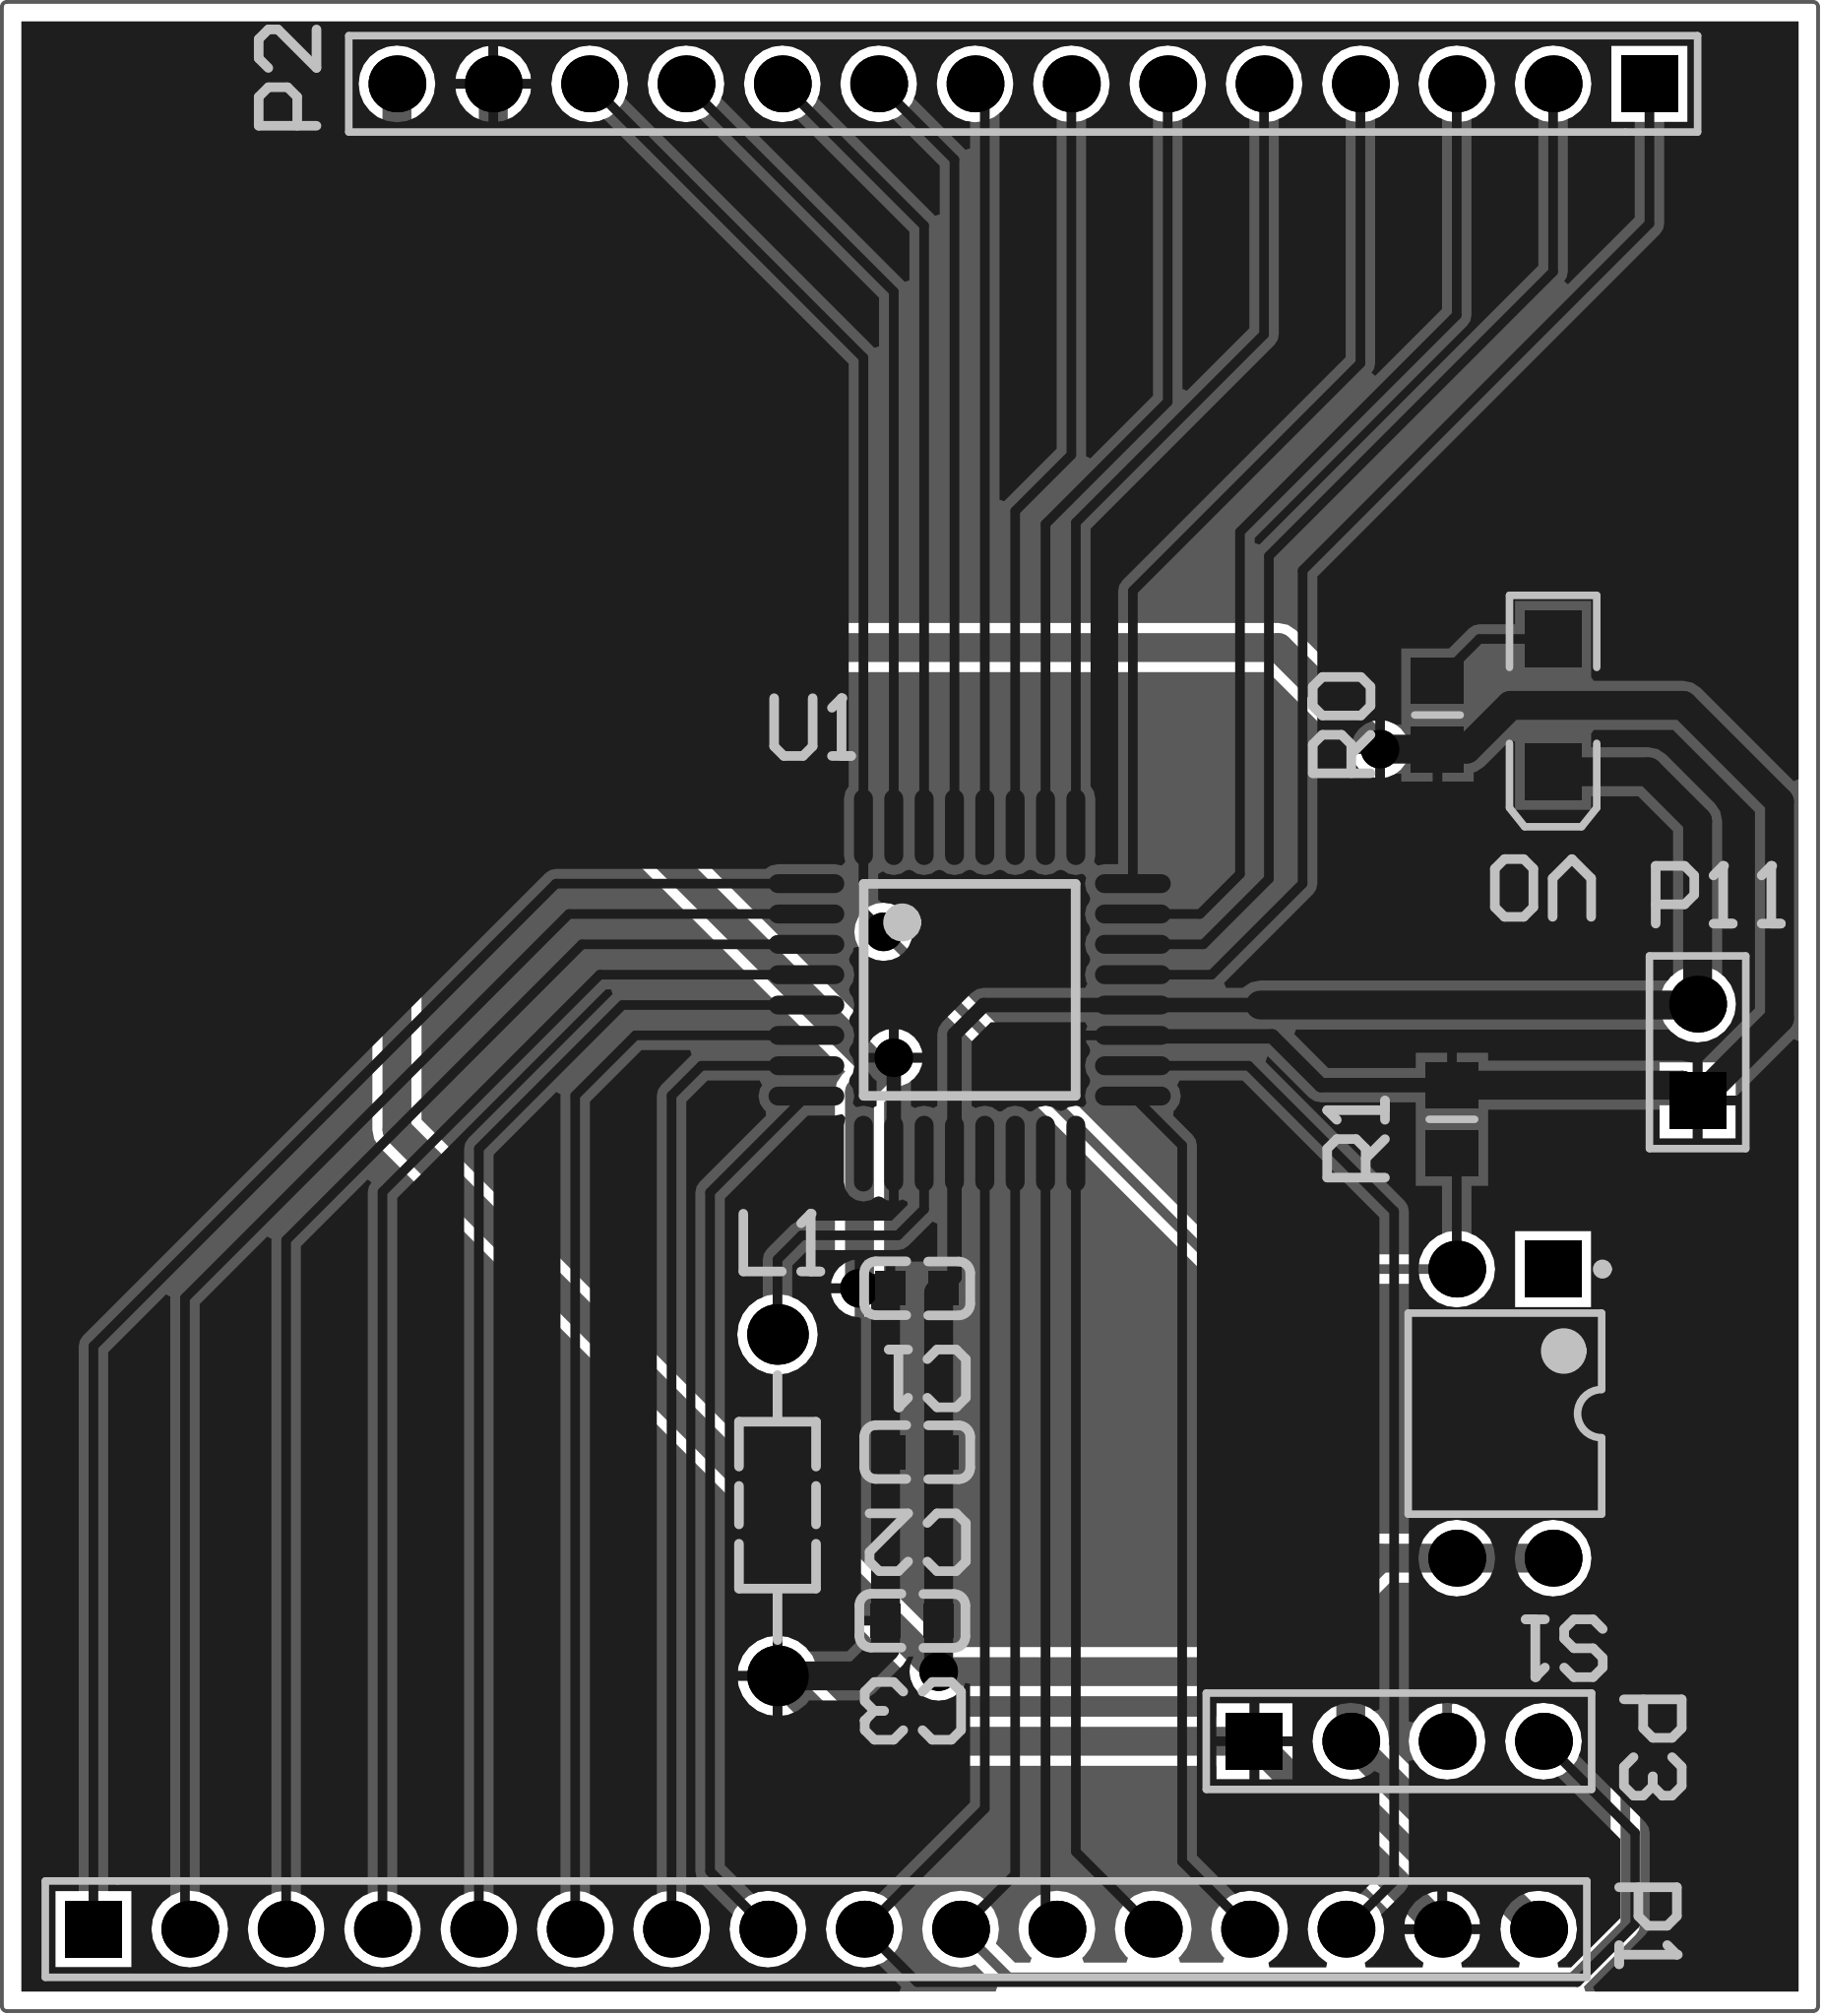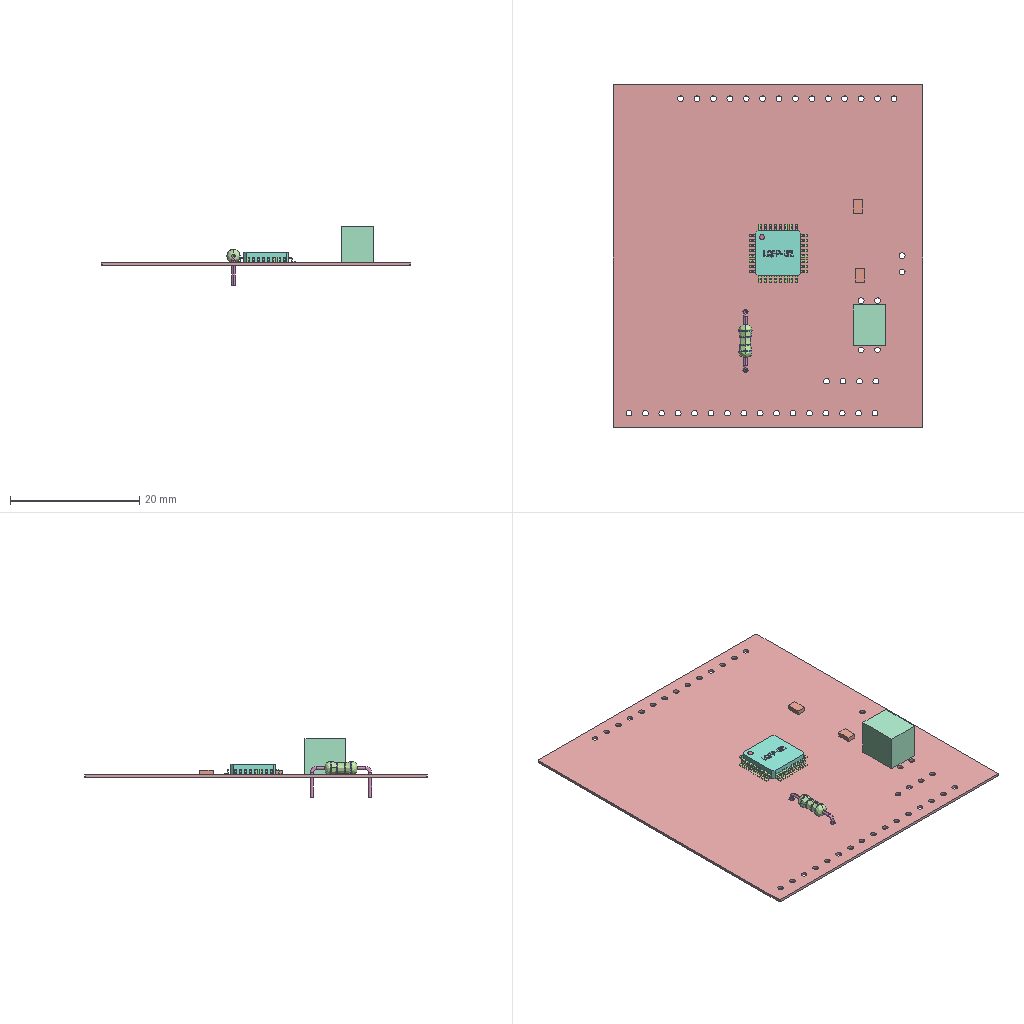Circuit board layout | Altium Designer | box 47.9 x 53 x 9.1 mm
Layer stack:
# Altium Designer layer stack of 2 (unit mm; dielectric type: 0 none, 1 core, 2 prepreg, 3 surface material)
index,name,kind,layer,copper_thickness_mm,dielectric_type,dielectric_thickness_mm,dielectric_material,dielectric_constant
0,Top Paste,other,,,,,,
1,Top Overlay,other,,,,,,
2,Top Solder,dielectric,,,3,0.0102,Solder Resist,3.5
3,Top Layer,copper,Top Layer,0.0356,,,,
4,Dielectric 1,dielectric,,,0,0.32,FR-4,4.8
5,Bottom Layer,copper,Bottom Layer,0.0356,,,,
6,Bottom Solder,dielectric,,,3,0.0102,Solder Resist,3.5
7,Bottom Overlay,other,,,,,,
8,Bottom Paste,other,,,,,,
# drill layer pairs: low layer,high layer
drill_pair,Top Layer,Bottom Layer
Part placement:
Designator,Comment,Layer,Footprint,Center-X(mm),Center-Y(mm),Rotation
V0,Red LED_0603,TopLayer,3.2X1.6X1.1,104.902,97.79,270
U1,STC15F2K60S2_QFP32,TopLayer,LQFP32,89.52,90.277,0
S1,DIP switch-2P,TopLayer,DIP-4,103.632,79.121,270
R1,10k,TopLayer,6-0805_N,102.235,86.879,90
R0,10K,TopLayer,6-0805_N,101.854,97.536,90
P11,HX25003-2WAG,TopLayer,HDR1X2,108.712,88.646,90
P3,Right-angle pin header-4P,TopLayer,HDR1X4,100.838,70.485,360
P2,Header 14,TopLayer,HDR1X14,90.932,114.173,180
P1,Header 16,TopLayer,HDR1X16,85.471,65.532,360
L1,GZ1608D601TF,TopLayer,AL0204,84.455,76.708,90
C3,22uF,TopLayer,C0603,88.003,73.663,180
C2,100nF,TopLayer,C0603,88.13,78.108,180
C1,100nF,TopLayer,C0603,88.13,82.426,180
Design rules, without the lines most boards share:
# Altium Designer design rules of 2 (exported by Altium Designer, unit mm)
# columns: name | kind | enabled | priority | scope1 | scope2 | descriptor | typed fields (field=value)
HoleToHoleClearance | 52 | enabled | 1 | All | All | Hole To Hole Clearance (Gap=10mil) (All),(All) | gap=0.254
DiffPairsRouting | 51 | enabled | 1 | All | All | Differential Pairs Uncoupled Length using the Gap Constraints (Min=10mil) (Max=10mil) (Prefered=10mil)  and Width Constraints (Min=15mil) (Max=15mil) (Prefered=15mil) (All) |
SolderMaskExpansion | 13 | enabled | 1 | All | All | Solder Mask Expansion (Expansion =4mil) (All) | expansion=0.1016
PasteMaskExpansion | 14 | enabled | 1 | All | All | Paste Mask Expansion (Expansion =0mil) (All) | expansion=0
RoutingVias | 11 | enabled | 1 | All | All | Routing Via (MinHoleWidth=28mil) (MaxHoleWidth=28mil) (PreferredHoleWidth=28mil) (MinWidth=50mil) (MaxWidth=50mil) (PreferedWidth=50mil) (All) | via_min_hole=0.7112 via_max_hole=0.7112 via_preferred_diameter=1.27 via_preferred_hole=0.7112
Width | 2 | enabled | 1 | All | All | Width Constraint (Min=10mil) (Max=10mil) (Preferred=10mil) (All) |
PolygonConnect | 20 | enabled | 1 | All | All | Polygon Connect Rule(Relief Connect )(Conductor Width=10mil) (Relief Angle=90 Angle) (Entries=4) (Air Gap Width=10mil) (All),(All) | connect_style(0=relief,1=direct,2=none)=0 relief_conductor_width=0.254 relief_entries=4
PlaneConnect | 6 | enabled | 1 | All | All | Power Plane Connect Rule(Relief Connect )(Expansion=20mil) (Conductor Width=10mil) (Air Gap=10mil) (Entries=4) (All) | relief_conductor_width=0.254 relief_entries=4 relief_expansion=0.508
Clearance | 0 | enabled | 1 | All | All | Clearance Constraint (Gap=10mil) (All),(All) | gap=0.254